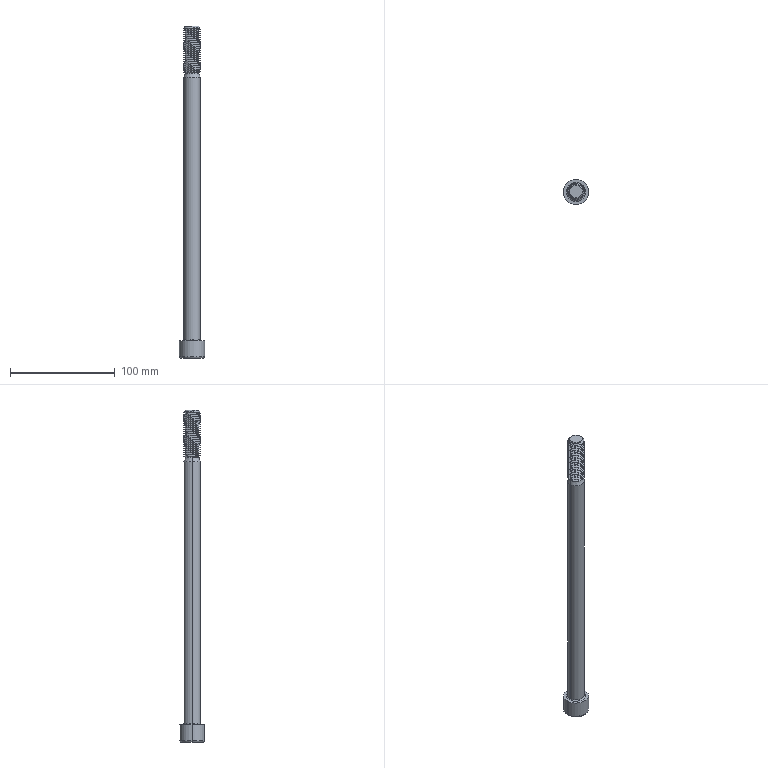Part | STEP file | Parafuso M16 - 300mm - DIN 912 (DIN EM ISO 4762) | 1 solid | 72 faces | box 24 x 24 x 316.5 mm | volume 64272 mm3 | cylinder 47 | plane 10 | cone 9 | torus 4 | spline 2 | commonest cylinder face diameters 16 x45 24 x2